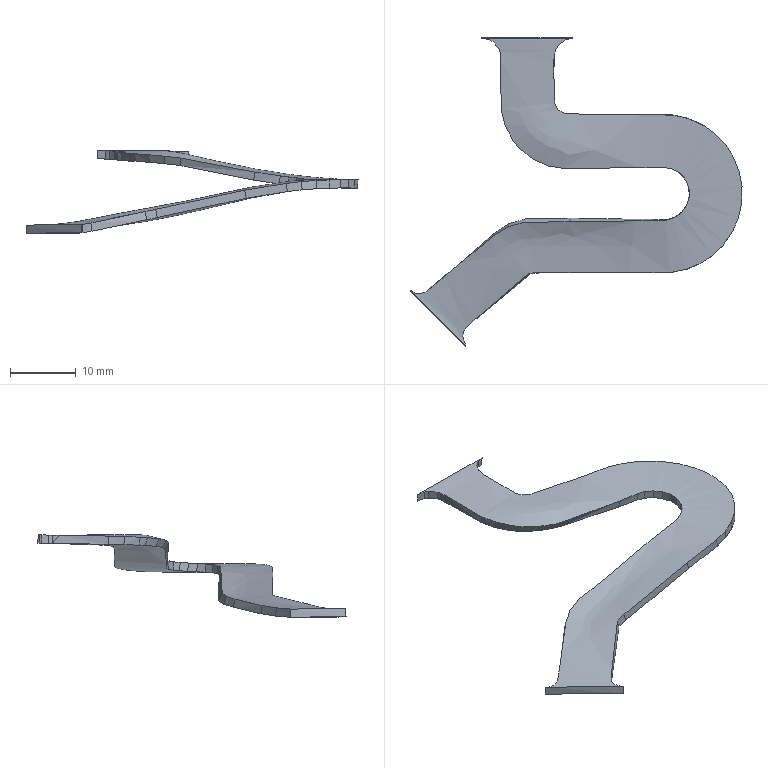Part | STEP file | gslz 2016.10.28-13_id1254_x_t | 1 solid | 67 faces | box 50.336 x 46.733 x 12.552 mm | volume 985.225 mm3 | spline 67